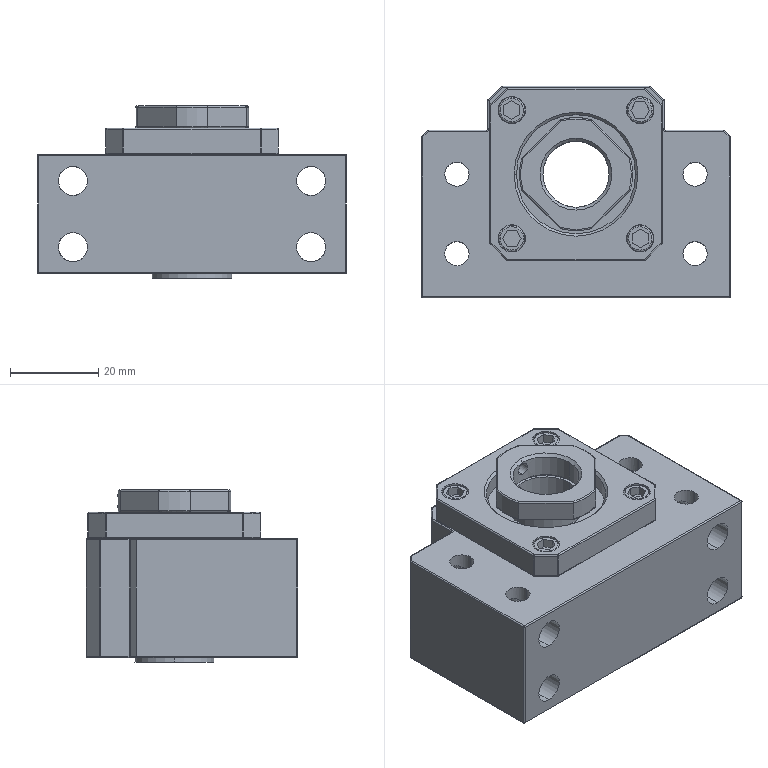Part | STEP file | 001-003-BK15 | 5 solids | 317 faces | box 70 x 48 x 39 mm | volume 76186 mm3 | cylinder 165 | plane 86 | spline 50 | cone 16 | commonest cylinder face diameters 0.56 x32 0.6 x32 5.5 x24 18 x10 5.88 x8 6.174 x8